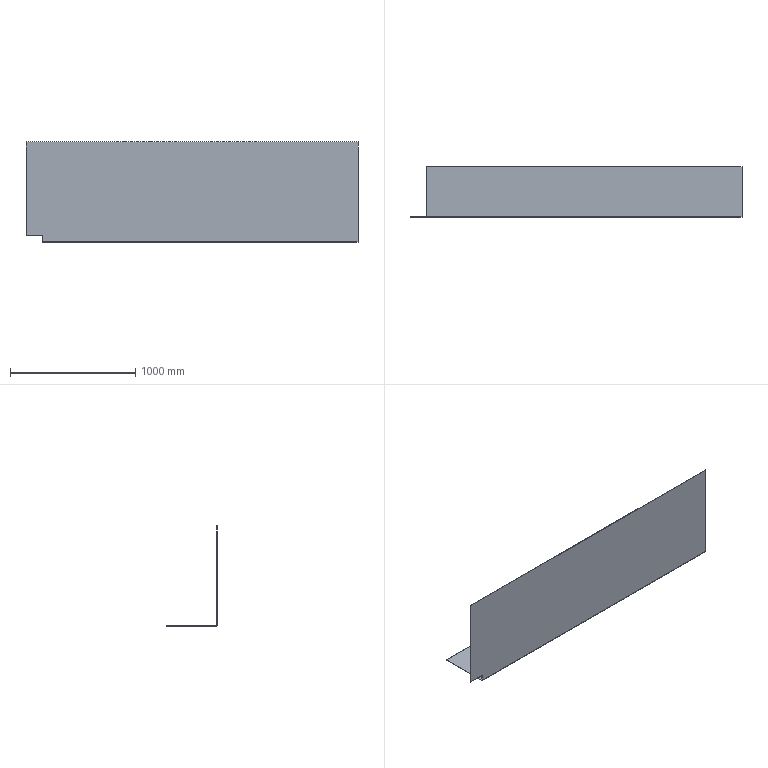Part | STEP file | E3-花纹Plate折弯1 | 1 solid | 14 faces | box 2648 x 403 x 798 mm | volume 9332526 mm3 | plane 12 | cylinder 2 | commonest cylinder face diameters 2 x1 8 x1
STEP:
#1=CARTESIAN_POINT('',(0.,0.,0.));
#2=DIRECTION('',(0.,0.,1.));
#3=DIRECTION('',(1.,0.,0.));
#4=AXIS2_PLACEMENT_3D('',#1,#2,#3);
#5=CARTESIAN_POINT('',(2648.,3.,-794.));
#6=VERTEX_POINT('',#5);
#7=CARTESIAN_POINT('',(2648.,3.,0.));
#8=VERTEX_POINT('',#7);
#9=CARTESIAN_POINT('',(2648.,3.,0.));
#10=DIRECTION('',(0.,0.,1.));
#11=VECTOR('',#10,1.);
#12=LINE('',#9,#11);
#13=CARTESIAN_POINT('',(2648.,3.,0.));
#14=DIRECTION('',(1.,0.,0.));
#15=DIRECTION('',(0.,0.,1.));
#16=AXIS2_PLACEMENT_3D('',#13,#14,#15);
#17=PLANE('',#16);
#18=CARTESIAN_POINT('',(0.,0.));
#19=DIRECTION('',(1.,0.));
#20=VECTOR('',#19,1.);
#21=LINE('',#18,#20);
#22=(GEOMETRIC_REPRESENTATION_CONTEXT(2)PARAMETRIC_REPRESENTATION_CONTEXT()REPRESENTATION_CONTEXT('',''));
#23=DEFINITIONAL_REPRESENTATION('',(#21),#22);
#24=PCURVE('',#17,#23);
#25=CARTESIAN_POINT('',(0.,3.,0.));
#26=DIRECTION('',(0.,1.,0.));
#27=DIRECTION('',(0.,0.,-1.));
#28=AXIS2_PLACEMENT_3D('',#25,#26,#27);
#29=PLANE('',#28);
#30=CARTESIAN_POINT('',(0.,-2648.));
#31=DIRECTION('',(-1.,0.));
#32=VECTOR('',#31,1.);
#33=LINE('',#30,#32);
#34=(GEOMETRIC_REPRESENTATION_CONTEXT(2)PARAMETRIC_REPRESENTATION_CONTEXT()REPRESENTATION_CONTEXT('',''));
#35=DEFINITIONAL_REPRESENTATION('',(#33),#34);
#36=PCURVE('',#29,#35);
#37=SURFACE_CURVE('',#12,(#24,#36),.PCURVE_S1.);
#38=EDGE_CURVE('',#6,#8,#37,.T.);
#39=ORIENTED_EDGE('',*,*,#38,.T.);
#40=CARTESIAN_POINT('',(2648.,0.,0.));
#41=VERTEX_POINT('',#40);
#42=CARTESIAN_POINT('',(2648.,3.,0.));
#43=DIRECTION('',(0.,1.,0.));
#44=VECTOR('',#43,1.);
#45=LINE('',#42,#44);
#46=CARTESIAN_POINT('',(0.,0.));
#47=DIRECTION('',(0.,-1.));
#48=VECTOR('',#47,1.);
#49=LINE('',#46,#48);
#50=(GEOMETRIC_REPRESENTATION_CONTEXT(2)PARAMETRIC_REPRESENTATION_CONTEXT()REPRESENTATION_CONTEXT('',''));
#51=DEFINITIONAL_REPRESENTATION('',(#49),#50);
#52=PCURVE('',#17,#51);
#53=CARTESIAN_POINT('',(0.,3.,0.));
#54=DIRECTION('',(0.,0.,1.));
#55=DIRECTION('',(-1.,0.,0.));
#56=AXIS2_PLACEMENT_3D('',#53,#54,#55);
#57=PLANE('',#56);
#58=CARTESIAN_POINT('',(-2648.,0.));
#59=DIRECTION('',(0.,-1.));
#60=VECTOR('',#59,1.);
#61=LINE('',#58,#60);
#62=(GEOMETRIC_REPRESENTATION_CONTEXT(2)PARAMETRIC_REPRESENTATION_CONTEXT()REPRESENTATION_CONTEXT('',''));
#63=DEFINITIONAL_REPRESENTATION('',(#61),#62);
#64=PCURVE('',#57,#63);
#65=SURFACE_CURVE('',#45,(#52,#64),.PCURVE_S1.);
#66=EDGE_CURVE('',#41,#8,#65,.T.);
#67=ORIENTED_EDGE('',*,*,#66,.F.);
#68=CARTESIAN_POINT('',(2648.,0.,-794.));
#69=VERTEX_POINT('',#68);
#70=CARTESIAN_POINT('',(2648.,0.,0.));
#71=DIRECTION('',(0.,0.,1.));
#72=VECTOR('',#71,1.);
#73=LINE('',#70,#72);
#74=CARTESIAN_POINT('',(0.,3.));
#75=DIRECTION('',(1.,0.));
#76=VECTOR('',#75,1.);
#77=LINE('',#74,#76);
#78=(GEOMETRIC_REPRESENTATION_CONTEXT(2)PARAMETRIC_REPRESENTATION_CONTEXT()REPRESENTATION_CONTEXT('',''));
#79=DEFINITIONAL_REPRESENTATION('',(#77),#78);
#80=PCURVE('',#17,#79);
#81=CARTESIAN_POINT('',(0.,0.,0.));
#82=DIRECTION('',(0.,1.,0.));
#83=DIRECTION('',(0.,0.,-1.));
#84=AXIS2_PLACEMENT_3D('',#81,#82,#83);
#85=PLANE('',#84);
#86=CARTESIAN_POINT('',(0.,-2648.));
#87=DIRECTION('',(-1.,0.));
#88=VECTOR('',#87,1.);
#89=LINE('',#86,#88);
#90=(GEOMETRIC_REPRESENTATION_CONTEXT(2)PARAMETRIC_REPRESENTATION_CONTEXT()REPRESENTATION_CONTEXT('',''));
#91=DEFINITIONAL_REPRESENTATION('',(#89),#90);
#92=PCURVE('',#85,#91);
#93=SURFACE_CURVE('',#73,(#80,#92),.PCURVE_S1.);
#94=EDGE_CURVE('',#69,#41,#93,.T.);
#95=ORIENTED_EDGE('',*,*,#94,.F.);
#96=CARTESIAN_POINT('',(2648.,3.,-794.));
#97=DIRECTION('',(0.,-1.,0.));
#98=VECTOR('',#97,1.);
#99=LINE('',#96,#98);
#100=CARTESIAN_POINT('',(-794.,0.));
#101=DIRECTION('',(0.,1.));
#102=VECTOR('',#101,1.);
#103=LINE('',#100,#102);
#104=(GEOMETRIC_REPRESENTATION_CONTEXT(2)PARAMETRIC_REPRESENTATION_CONTEXT()REPRESENTATION_CONTEXT('',''));
#105=DEFINITIONAL_REPRESENTATION('',(#103),#104);
#106=PCURVE('',#17,#105);
#107=CARTESIAN_POINT('',(2648.,4.,-794.));
#108=DIRECTION('',(-1.,0.,0.));
#109=DIRECTION('',(0.,0.,-1.));
#110=AXIS2_PLACEMENT_3D('',#107,#108,#109);
#111=PLANE('',#110);
#112=CARTESIAN_POINT('',(0.,1.));
#113=DIRECTION('',(0.,1.));
#114=VECTOR('',#113,1.);
#115=LINE('',#112,#114);
#116=(GEOMETRIC_REPRESENTATION_CONTEXT(2)PARAMETRIC_REPRESENTATION_CONTEXT()REPRESENTATION_CONTEXT('',''));
#117=DEFINITIONAL_REPRESENTATION('',(#115),#116);
#118=PCURVE('',#111,#117);
#119=SURFACE_CURVE('',#99,(#106,#118),.PCURVE_S1.);
#120=EDGE_CURVE('',#6,#69,#119,.T.);
#121=ORIENTED_EDGE('',*,*,#120,.F.);
#122=EDGE_LOOP('',(#39,#67,#95,#121));
#123=FACE_BOUND('',#122,.T.);
#124=ADVANCED_FACE('',(#123),#17,.T.);
#125=CARTESIAN_POINT('',(130.,3.,-746.));
#126=VERTEX_POINT('',#125);
#127=CARTESIAN_POINT('',(0.,3.,-746.));
#128=VERTEX_POINT('',#127);
#129=CARTESIAN_POINT('',(0.,3.,-746.));
#130=DIRECTION('',(-1.,0.,0.));
#131=VECTOR('',#130,1.);
#132=LINE('',#129,#131);
#133=CARTESIAN_POINT('',(746.,0.));
#134=DIRECTION('',(0.,1.));
#135=VECTOR('',#134,1.);
#136=LINE('',#133,#135);
#137=(GEOMETRIC_REPRESENTATION_CONTEXT(2)PARAMETRIC_REPRESENTATION_CONTEXT()REPRESENTATION_CONTEXT('',''));
#138=DEFINITIONAL_REPRESENTATION('',(#136),#137);
#139=PCURVE('',#29,#138);
#140=CARTESIAN_POINT('',(0.,-497.,-746.));
#141=DIRECTION('',(0.,0.,1.));
#142=DIRECTION('',(-1.,0.,0.));
#143=AXIS2_PLACEMENT_3D('',#140,#141,#142);
#144=PLANE('',#143);
#145=CARTESIAN_POINT('',(0.,-500.));
#146=DIRECTION('',(1.,0.));
#147=VECTOR('',#146,1.);
#148=LINE('',#145,#147);
#149=(GEOMETRIC_REPRESENTATION_CONTEXT(2)PARAMETRIC_REPRESENTATION_CONTEXT()REPRESENTATION_CONTEXT('',''));
#150=DEFINITIONAL_REPRESENTATION('',(#148),#149);
#151=PCURVE('',#144,#150);
#152=SURFACE_CURVE('',#132,(#139,#151),.PCURVE_S1.);
#153=EDGE_CURVE('',#126,#128,#152,.T.);
#154=ORIENTED_EDGE('',*,*,#153,.T.);
#155=CARTESIAN_POINT('',(0.,3.,0.));
#156=VERTEX_POINT('',#155);
#157=CARTESIAN_POINT('',(0.,3.,0.));
#158=DIRECTION('',(0.,0.,-1.));
#159=VECTOR('',#158,1.);
#160=LINE('',#157,#159);
#161=CARTESIAN_POINT('',(0.,0.));
#162=DIRECTION('',(1.,0.));
#163=VECTOR('',#162,1.);
#164=LINE('',#161,#163);
#165=(GEOMETRIC_REPRESENTATION_CONTEXT(2)PARAMETRIC_REPRESENTATION_CONTEXT()REPRESENTATION_CONTEXT('',''));
#166=DEFINITIONAL_REPRESENTATION('',(#164),#165);
#167=PCURVE('',#29,#166);
#168=CARTESIAN_POINT('',(0.,3.,0.));
#169=DIRECTION('',(-1.,0.,0.));
#170=DIRECTION('',(0.,0.,-1.));
#171=AXIS2_PLACEMENT_3D('',#168,#169,#170);
#172=PLANE('',#171);
#173=CARTESIAN_POINT('',(0.,0.));
#174=DIRECTION('',(1.,0.));
#175=VECTOR('',#174,1.);
#176=LINE('',#173,#175);
#177=(GEOMETRIC_REPRESENTATION_CONTEXT(2)PARAMETRIC_REPRESENTATION_CONTEXT()REPRESENTATION_CONTEXT('',''));
#178=DEFINITIONAL_REPRESENTATION('',(#176),#177);
#179=PCURVE('',#172,#178);
#180=SURFACE_CURVE('',#160,(#167,#179),.PCURVE_S1.);
#181=EDGE_CURVE('',#156,#128,#180,.T.);
#182=ORIENTED_EDGE('',*,*,#181,.F.);
#183=CARTESIAN_POINT('',(0.,3.,0.));
#184=DIRECTION('',(-1.,0.,0.));
#185=VECTOR('',#184,1.);
#186=LINE('',#183,#185);
#187=CARTESIAN_POINT('',(0.,0.));
#188=DIRECTION('',(0.,1.));
#189=VECTOR('',#188,1.);
#190=LINE('',#187,#189);
#191=(GEOMETRIC_REPRESENTATION_CONTEXT(2)PARAMETRIC_REPRESENTATION_CONTEXT()REPRESENTATION_CONTEXT('',''));
#192=DEFINITIONAL_REPRESENTATION('',(#190),#191);
#193=PCURVE('',#29,#192);
#194=CARTESIAN_POINT('',(0.,0.));
#195=DIRECTION('',(1.,0.));
#196=VECTOR('',#195,1.);
#197=LINE('',#194,#196);
#198=(GEOMETRIC_REPRESENTATION_CONTEXT(2)PARAMETRIC_REPRESENTATION_CONTEXT()REPRESENTATION_CONTEXT('',''));
#199=DEFINITIONAL_REPRESENTATION('',(#197),#198);
#200=PCURVE('',#57,#199);
#201=SURFACE_CURVE('',#186,(#193,#200),.PCURVE_S1.);
#202=EDGE_CURVE('',#8,#156,#201,.T.);
#203=ORIENTED_EDGE('',*,*,#202,.F.);
#204=ORIENTED_EDGE('',*,*,#38,.F.);
#205=CARTESIAN_POINT('',(130.,3.,-794.));
#206=VERTEX_POINT('',#205);
#207=CARTESIAN_POINT('',(2648.,3.,-794.));
#208=DIRECTION('',(-1.,0.,0.));
#209=VECTOR('',#208,1.);
#210=LINE('',#207,#209);
#211=CARTESIAN_POINT('',(794.,-2648.));
#212=DIRECTION('',(0.,1.));
#213=VECTOR('',#212,1.);
#214=LINE('',#211,#213);
#215=(GEOMETRIC_REPRESENTATION_CONTEXT(2)PARAMETRIC_REPRESENTATION_CONTEXT()REPRESENTATION_CONTEXT('',''));
#216=DEFINITIONAL_REPRESENTATION('',(#214),#215);
#217=PCURVE('',#29,#216);
#218=CARTESIAN_POINT('',(2648.,4.,-794.));
#219=DIRECTION('',(1.,0.,0.));
#220=DIRECTION('',(0.,0.,-1.));
#221=AXIS2_PLACEMENT_3D('',#218,#219,#220);
#222=CYLINDRICAL_SURFACE('',#221,1.);
#223=CARTESIAN_POINT('',(4.712,0.));
#224=DIRECTION('',(0.,-1.));
#225=VECTOR('',#224,1.);
#226=LINE('',#223,#225);
#227=(GEOMETRIC_REPRESENTATION_CONTEXT(2)PARAMETRIC_REPRESENTATION_CONTEXT()REPRESENTATION_CONTEXT('',''));
#228=DEFINITIONAL_REPRESENTATION('',(#226),#227);
#229=PCURVE('',#222,#228);
#230=SURFACE_CURVE('',#210,(#217,#229),.PCURVE_S1.);
#231=EDGE_CURVE('',#6,#206,#230,.T.);
#232=ORIENTED_EDGE('',*,*,#231,.T.);
#233=CARTESIAN_POINT('',(130.,3.,0.));
#234=DIRECTION('',(0.,0.,1.));
#235=VECTOR('',#234,1.);
#236=LINE('',#233,#235);
#237=CARTESIAN_POINT('',(0.,-130.));
#238=DIRECTION('',(-1.,0.));
#239=VECTOR('',#238,1.);
#240=LINE('',#237,#239);
#241=(GEOMETRIC_REPRESENTATION_CONTEXT(2)PARAMETRIC_REPRESENTATION_CONTEXT()REPRESENTATION_CONTEXT('',''));
#242=DEFINITIONAL_REPRESENTATION('',(#240),#241);
#243=PCURVE('',#29,#242);
#244=CARTESIAN_POINT('',(130.,-497.,-746.));
#245=DIRECTION('',(1.,0.,0.));
#246=DIRECTION('',(0.,0.,1.));
#247=AXIS2_PLACEMENT_3D('',#244,#245,#246);
#248=PLANE('',#247);
#249=CARTESIAN_POINT('',(746.,-500.));
#250=DIRECTION('',(1.,0.));
#251=VECTOR('',#250,1.);
#252=LINE('',#249,#251);
#253=(GEOMETRIC_REPRESENTATION_CONTEXT(2)PARAMETRIC_REPRESENTATION_CONTEXT()REPRESENTATION_CONTEXT('',''));
#254=DEFINITIONAL_REPRESENTATION('',(#252),#253);
#255=PCURVE('',#248,#254);
#256=SURFACE_CURVE('',#236,(#243,#255),.PCURVE_S1.);
#257=EDGE_CURVE('',#206,#126,#256,.T.);
#258=ORIENTED_EDGE('',*,*,#257,.T.);
#259=EDGE_LOOP('',(#154,#182,#203,#204,#232,#258));
#260=FACE_BOUND('',#259,.T.);
#261=ADVANCED_FACE('',(#260),#29,.T.);
#262=CARTESIAN_POINT('',(130.,0.,-794.));
#263=VERTEX_POINT('',#262);
#264=CARTESIAN_POINT('',(130.,0.,-746.));
#265=VERTEX_POINT('',#264);
#266=CARTESIAN_POINT('',(130.,0.,0.));
#267=DIRECTION('',(0.,0.,1.));
#268=VECTOR('',#267,1.);
#269=LINE('',#266,#268);
#270=CARTESIAN_POINT('',(0.,-130.));
#271=DIRECTION('',(-1.,0.));
#272=VECTOR('',#271,1.);
#273=LINE('',#270,#272);
#274=(GEOMETRIC_REPRESENTATION_CONTEXT(2)PARAMETRIC_REPRESENTATION_CONTEXT()REPRESENTATION_CONTEXT('',''));
#275=DEFINITIONAL_REPRESENTATION('',(#273),#274);
#276=PCURVE('',#85,#275);
#277=CARTESIAN_POINT('',(746.,-497.));
#278=DIRECTION('',(1.,0.));
#279=VECTOR('',#278,1.);
#280=LINE('',#277,#279);
#281=(GEOMETRIC_REPRESENTATION_CONTEXT(2)PARAMETRIC_REPRESENTATION_CONTEXT()REPRESENTATION_CONTEXT('',''));
#282=DEFINITIONAL_REPRESENTATION('',(#280),#281);
#283=PCURVE('',#248,#282);
#284=SURFACE_CURVE('',#269,(#276,#283),.PCURVE_S1.);
#285=EDGE_CURVE('',#263,#265,#284,.T.);
#286=ORIENTED_EDGE('',*,*,#285,.F.);
#287=CARTESIAN_POINT('',(2648.,0.,-794.));
#288=DIRECTION('',(-1.,0.,0.));
#289=VECTOR('',#288,1.);
#290=LINE('',#287,#289);
#291=CARTESIAN_POINT('',(794.,-2648.));
#292=DIRECTION('',(0.,1.));
#293=VECTOR('',#292,1.);
#294=LINE('',#291,#293);
#295=(GEOMETRIC_REPRESENTATION_CONTEXT(2)PARAMETRIC_REPRESENTATION_CONTEXT()REPRESENTATION_CONTEXT('',''));
#296=DEFINITIONAL_REPRESENTATION('',(#294),#295);
#297=PCURVE('',#85,#296);
#298=CARTESIAN_POINT('',(2648.,4.,-794.));
#299=DIRECTION('',(1.,0.,0.));
#300=DIRECTION('',(0.,0.,-1.));
#301=AXIS2_PLACEMENT_3D('',#298,#299,#300);
#302=CYLINDRICAL_SURFACE('',#301,4.);
#303=CARTESIAN_POINT('',(4.712,0.));
#304=DIRECTION('',(0.,-1.));
#305=VECTOR('',#304,1.);
#306=LINE('',#303,#305);
#307=(GEOMETRIC_REPRESENTATION_CONTEXT(2)PARAMETRIC_REPRESENTATION_CONTEXT()REPRESENTATION_CONTEXT('',''));
#308=DEFINITIONAL_REPRESENTATION('',(#306),#307);
#309=PCURVE('',#302,#308);
#310=SURFACE_CURVE('',#290,(#297,#309),.PCURVE_S1.);
#311=EDGE_CURVE('',#69,#263,#310,.T.);
#312=ORIENTED_EDGE('',*,*,#311,.F.);
#313=ORIENTED_EDGE('',*,*,#94,.T.);
#314=CARTESIAN_POINT('',(0.,0.,0.));
#315=VERTEX_POINT('',#314);
#316=CARTESIAN_POINT('',(0.,0.,0.));
#317=DIRECTION('',(-1.,0.,0.));
#318=VECTOR('',#317,1.);
#319=LINE('',#316,#318);
#320=CARTESIAN_POINT('',(0.,0.));
#321=DIRECTION('',(0.,1.));
#322=VECTOR('',#321,1.);
#323=LINE('',#320,#322);
#324=(GEOMETRIC_REPRESENTATION_CONTEXT(2)PARAMETRIC_REPRESENTATION_CONTEXT()REPRESENTATION_CONTEXT('',''));
#325=DEFINITIONAL_REPRESENTATION('',(#323),#324);
#326=PCURVE('',#85,#325);
#327=CARTESIAN_POINT('',(0.,3.));
#328=DIRECTION('',(1.,0.));
#329=VECTOR('',#328,1.);
#330=LINE('',#327,#329);
#331=(GEOMETRIC_REPRESENTATION_CONTEXT(2)PARAMETRIC_REPRESENTATION_CONTEXT()REPRESENTATION_CONTEXT('',''));
#332=DEFINITIONAL_REPRESENTATION('',(#330),#331);
#333=PCURVE('',#57,#332);
#334=SURFACE_CURVE('',#319,(#326,#333),.PCURVE_S1.);
#335=EDGE_CURVE('',#41,#315,#334,.T.);
#336=ORIENTED_EDGE('',*,*,#335,.T.);
#337=CARTESIAN_POINT('',(0.,0.,-746.));
#338=VERTEX_POINT('',#337);
#339=CARTESIAN_POINT('',(0.,0.,0.));
#340=DIRECTION('',(0.,0.,-1.));
#341=VECTOR('',#340,1.);
#342=LINE('',#339,#341);
#343=CARTESIAN_POINT('',(0.,0.));
#344=DIRECTION('',(1.,0.));
#345=VECTOR('',#344,1.);
#346=LINE('',#343,#345);
#347=(GEOMETRIC_REPRESENTATION_CONTEXT(2)PARAMETRIC_REPRESENTATION_CONTEXT()REPRESENTATION_CONTEXT('',''));
#348=DEFINITIONAL_REPRESENTATION('',(#346),#347);
#349=PCURVE('',#85,#348);
#350=CARTESIAN_POINT('',(0.,3.));
#351=DIRECTION('',(1.,0.));
#352=VECTOR('',#351,1.);
#353=LINE('',#350,#352);
#354=(GEOMETRIC_REPRESENTATION_CONTEXT(2)PARAMETRIC_REPRESENTATION_CONTEXT()REPRESENTATION_CONTEXT('',''));
#355=DEFINITIONAL_REPRESENTATION('',(#353),#354);
#356=PCURVE('',#172,#355);
#357=SURFACE_CURVE('',#342,(#349,#356),.PCURVE_S1.);
#358=EDGE_CURVE('',#315,#338,#357,.T.);
#359=ORIENTED_EDGE('',*,*,#358,.T.);
#360=CARTESIAN_POINT('',(0.,0.,-746.));
#361=DIRECTION('',(-1.,0.,0.));
#362=VECTOR('',#361,1.);
#363=LINE('',#360,#362);
#364=CARTESIAN_POINT('',(746.,0.));
#365=DIRECTION('',(0.,1.));
#366=VECTOR('',#365,1.);
#367=LINE('',#364,#366);
#368=(GEOMETRIC_REPRESENTATION_CONTEXT(2)PARAMETRIC_REPRESENTATION_CONTEXT()REPRESENTATION_CONTEXT('',''));
#369=DEFINITIONAL_REPRESENTATION('',(#367),#368);
#370=PCURVE('',#85,#369);
#371=CARTESIAN_POINT('',(0.,-497.));
#372=DIRECTION('',(1.,0.));
#373=VECTOR('',#372,1.);
#374=LINE('',#371,#373);
#375=(GEOMETRIC_REPRESENTATION_CONTEXT(2)PARAMETRIC_REPRESENTATION_CONTEXT()REPRESENTATION_CONTEXT('',''));
#376=DEFINITIONAL_REPRESENTATION('',(#374),#375);
#377=PCURVE('',#144,#376);
#378=SURFACE_CURVE('',#363,(#370,#377),.PCURVE_S1.);
#379=EDGE_CURVE('',#265,#338,#378,.T.);
#380=ORIENTED_EDGE('',*,*,#379,.F.);
#381=EDGE_LOOP('',(#286,#312,#313,#336,#359,#380));
#382=FACE_BOUND('',#381,.T.);
#383=ADVANCED_FACE('',(#382),#85,.F.);
#384=ORIENTED_EDGE('',*,*,#66,.T.);
#385=ORIENTED_EDGE('',*,*,#202,.T.);
#386=CARTESIAN_POINT('',(0.,3.,0.));
#387=DIRECTION('',(0.,1.,0.));
#388=VECTOR('',#387,1.);
#389=LINE('',#386,#388);
#390=CARTESIAN_POINT('',(0.,0.));
#391=DIRECTION('',(0.,-1.));
#392=VECTOR('',#391,1.);
#393=LINE('',#390,#392);
#394=(GEOMETRIC_REPRESENTATION_CONTEXT(2)PARAMETRIC_REPRESENTATION_CONTEXT()REPRESENTATION_CONTEXT('',''));
#395=DEFINITIONAL_REPRESENTATION('',(#393),#394);
#396=PCURVE('',#57,#395);
#397=CARTESIAN_POINT('',(0.,0.));
#398=DIRECTION('',(0.,-1.));
#399=VECTOR('',#398,1.);
#400=LINE('',#397,#399);
#401=(GEOMETRIC_REPRESENTATION_CONTEXT(2)PARAMETRIC_REPRESENTATION_CONTEXT()REPRESENTATION_CONTEXT('',''));
#402=DEFINITIONAL_REPRESENTATION('',(#400),#401);
#403=PCURVE('',#172,#402);
#404=SURFACE_CURVE('',#389,(#396,#403),.PCURVE_S1.);
#405=EDGE_CURVE('',#315,#156,#404,.T.);
#406=ORIENTED_EDGE('',*,*,#405,.F.);
#407=ORIENTED_EDGE('',*,*,#335,.F.);
#408=EDGE_LOOP('',(#384,#385,#406,#407));
#409=FACE_BOUND('',#408,.T.);
#410=ADVANCED_FACE('',(#409),#57,.T.);
#411=CARTESIAN_POINT('',(0.,-497.,-746.));
#412=DIRECTION('',(0.,1.,0.));
#413=VECTOR('',#412,1.);
#414=LINE('',#411,#413);
#415=CARTESIAN_POINT('',(746.,500.));
#416=DIRECTION('',(0.,-1.));
#417=VECTOR('',#416,1.);
#418=LINE('',#415,#417);
#419=(GEOMETRIC_REPRESENTATION_CONTEXT(2)PARAMETRIC_REPRESENTATION_CONTEXT()REPRESENTATION_CONTEXT('',''));
#420=DEFINITIONAL_REPRESENTATION('',(#418),#419);
#421=PCURVE('',#172,#420);
#422=CARTESIAN_POINT('',(0.,0.));
#423=DIRECTION('',(0.,-1.));
#424=VECTOR('',#423,1.);
#425=LINE('',#422,#424);
#426=(GEOMETRIC_REPRESENTATION_CONTEXT(2)PARAMETRIC_REPRESENTATION_CONTEXT()REPRESENTATION_CONTEXT('',''));
#427=DEFINITIONAL_REPRESENTATION('',(#425),#426);
#428=PCURVE('',#144,#427);
#429=SURFACE_CURVE('',#414,(#421,#428),.PCURVE_S1.);
#430=EDGE_CURVE('',#338,#128,#429,.T.);
#431=ORIENTED_EDGE('',*,*,#430,.F.);
#432=ORIENTED_EDGE('',*,*,#358,.F.);
#433=ORIENTED_EDGE('',*,*,#405,.T.);
#434=ORIENTED_EDGE('',*,*,#181,.T.);
#435=EDGE_LOOP('',(#431,#432,#433,#434));
#436=FACE_BOUND('',#435,.T.);
#437=ADVANCED_FACE('',(#436),#172,.T.);
#438=CARTESIAN_POINT('',(2648.,4.,-795.));
#439=VERTEX_POINT('',#438);
#440=CARTESIAN_POINT('',(2648.,4.,-794.));
#441=DIRECTION('',(-1.,0.,0.));
#442=DIRECTION('',(0.,0.,1.));
#443=AXIS2_PLACEMENT_3D('',#440,#441,#442);
#444=CIRCLE('',#443,1.);
#445=CARTESIAN_POINT('',(0.,0.));
#446=DIRECTION('',(-1.,0.));
#447=AXIS2_PLACEMENT_2D('',#445,#446);
#448=CIRCLE('',#447,1.);
#449=(GEOMETRIC_REPRESENTATION_CONTEXT(2)PARAMETRIC_REPRESENTATION_CONTEXT()REPRESENTATION_CONTEXT('',''));
#450=DEFINITIONAL_REPRESENTATION('',(#448),#449);
#451=PCURVE('',#111,#450);
#452=CARTESIAN_POINT('',(9.425,0.));
#453=DIRECTION('',(-1.,0.));
#454=VECTOR('',#453,1.);
#455=LINE('',#452,#454);
#456=(GEOMETRIC_REPRESENTATION_CONTEXT(2)PARAMETRIC_REPRESENTATION_CONTEXT()REPRESENTATION_CONTEXT('',''));
#457=DEFINITIONAL_REPRESENTATION('',(#455),#456);
#458=PCURVE('',#222,#457);
#459=SURFACE_CURVE('',#444,(#451,#458),.PCURVE_S1.);
#460=EDGE_CURVE('',#439,#6,#459,.T.);
#461=ORIENTED_EDGE('',*,*,#460,.T.);
#462=ORIENTED_EDGE('',*,*,#120,.T.);
#463=CARTESIAN_POINT('',(2648.,4.,-798.));
#464=VERTEX_POINT('',#463);
#465=CARTESIAN_POINT('',(2648.,4.,-794.));
#466=DIRECTION('',(-1.,0.,0.));
#467=DIRECTION('',(0.,0.,1.));
#468=AXIS2_PLACEMENT_3D('',#465,#466,#467);
#469=CIRCLE('',#468,4.);
#470=CARTESIAN_POINT('',(0.,0.));
#471=DIRECTION('',(-1.,0.));
#472=AXIS2_PLACEMENT_2D('',#470,#471);
#473=CIRCLE('',#472,4.);
#474=(GEOMETRIC_REPRESENTATION_CONTEXT(2)PARAMETRIC_REPRESENTATION_CONTEXT()REPRESENTATION_CONTEXT('',''));
#475=DEFINITIONAL_REPRESENTATION('',(#473),#474);
#476=PCURVE('',#111,#475);
#477=CARTESIAN_POINT('',(9.425,0.));
#478=DIRECTION('',(-1.,0.));
#479=VECTOR('',#478,1.);
#480=LINE('',#477,#479);
#481=(GEOMETRIC_REPRESENTATION_CONTEXT(2)PARAMETRIC_REPRESENTATION_CONTEXT()REPRESENTATION_CONTEXT('',''));
#482=DEFINITIONAL_REPRESENTATION('',(#480),#481);
#483=PCURVE('',#302,#482);
#484=SURFACE_CURVE('',#469,(#476,#483),.PCURVE_S1.);
#485=EDGE_CURVE('',#464,#69,#484,.T.);
#486=ORIENTED_EDGE('',*,*,#485,.F.);
#487=CARTESIAN_POINT('',(2648.,4.,-795.));
#488=DIRECTION('',(0.,0.,-1.));
#489=VECTOR('',#488,1.);
#490=LINE('',#487,#489);
#491=CARTESIAN_POINT('',(1.,0.));
#492=DIRECTION('',(1.,0.));
#493=VECTOR('',#492,1.);
#494=LINE('',#491,#493);
#495=(GEOMETRIC_REPRESENTATION_CONTEXT(2)PARAMETRIC_REPRESENTATION_CONTEXT()REPRESENTATION_CONTEXT('',''));
#496=DEFINITIONAL_REPRESENTATION('',(#494),#495);
#497=PCURVE('',#111,#496);
#498=CARTESIAN_POINT('',(2648.,403.,-798.));
#499=DIRECTION('',(-1.,0.,0.));
#500=DIRECTION('',(0.,0.,-1.));
#501=AXIS2_PLACEMENT_3D('',#498,#499,#500);
#502=PLANE('',#501);
#503=CARTESIAN_POINT('',(-3.,399.));
#504=DIRECTION('',(1.,0.));
#505=VECTOR('',#504,1.);
#506=LINE('',#503,#505);
#507=(GEOMETRIC_REPRESENTATION_CONTEXT(2)PARAMETRIC_REPRESENTATION_CONTEXT()REPRESENTATION_CONTEXT('',''));
#508=DEFINITIONAL_REPRESENTATION('',(#506),#507);
#509=PCURVE('',#502,#508);
#510=SURFACE_CURVE('',#490,(#497,#509),.PCURVE_S1.);
#511=EDGE_CURVE('',#439,#464,#510,.T.);
#512=ORIENTED_EDGE('',*,*,#511,.F.);
#513=EDGE_LOOP('',(#461,#462,#486,#512));
#514=FACE_BOUND('',#513,.T.);
#515=ADVANCED_FACE('',(#514),#111,.F.);
#516=CARTESIAN_POINT('',(130.,4.,-798.));
#517=VERTEX_POINT('',#516);
#518=CARTESIAN_POINT('',(130.,4.,-794.));
#519=DIRECTION('',(1.,0.,0.));
#520=DIRECTION('',(0.,0.,1.));
#521=AXIS2_PLACEMENT_3D('',#518,#519,#520);
#522=CIRCLE('',#521,4.);
#523=CARTESIAN_POINT('',(3.142,-2518.));
#524=DIRECTION('',(1.,0.));
#525=VECTOR('',#524,1.);
#526=LINE('',#523,#525);
#527=(GEOMETRIC_REPRESENTATION_CONTEXT(2)PARAMETRIC_REPRESENTATION_CONTEXT()REPRESENTATION_CONTEXT('',''));
#528=DEFINITIONAL_REPRESENTATION('',(#526),#527);
#529=PCURVE('',#302,#528);
#530=CARTESIAN_POINT('',(-48.,-501.));
#531=DIRECTION('',(1.,0.));
#532=AXIS2_PLACEMENT_2D('',#530,#531);
#533=CIRCLE('',#532,4.);
#534=(GEOMETRIC_REPRESENTATION_CONTEXT(2)PARAMETRIC_REPRESENTATION_CONTEXT()REPRESENTATION_CONTEXT('',''));
#535=DEFINITIONAL_REPRESENTATION('',(#533),#534);
#536=PCURVE('',#248,#535);
#537=SURFACE_CURVE('',#522,(#529,#536),.PCURVE_S1.);
#538=EDGE_CURVE('',#263,#517,#537,.T.);
#539=ORIENTED_EDGE('',*,*,#538,.T.);
#540=CARTESIAN_POINT('',(0.,4.,-798.));
#541=DIRECTION('',(-1.,0.,0.));
#542=VECTOR('',#541,1.);
#543=LINE('',#540,#542);
#544=CARTESIAN_POINT('',(6.283,-2648.));
#545=DIRECTION('',(0.,-1.));
#546=VECTOR('',#545,1.);
#547=LINE('',#544,#546);
#548=(GEOMETRIC_REPRESENTATION_CONTEXT(2)PARAMETRIC_REPRESENTATION_CONTEXT()REPRESENTATION_CONTEXT('',''));
#549=DEFINITIONAL_REPRESENTATION('',(#547),#548);
#550=PCURVE('',#302,#549);
#551=CARTESIAN_POINT('',(0.,0.,-798.));
#552=DIRECTION('',(0.,0.,1.));
#553=DIRECTION('',(-1.,0.,0.));
#554=AXIS2_PLACEMENT_3D('',#551,#552,#553);
#555=PLANE('',#554);
#556=CARTESIAN_POINT('',(0.,-4.));
#557=DIRECTION('',(1.,0.));
#558=VECTOR('',#557,1.);
#559=LINE('',#556,#558);
#560=(GEOMETRIC_REPRESENTATION_CONTEXT(2)PARAMETRIC_REPRESENTATION_CONTEXT()REPRESENTATION_CONTEXT('',''));
#561=DEFINITIONAL_REPRESENTATION('',(#559),#560);
#562=PCURVE('',#555,#561);
#563=SURFACE_CURVE('',#543,(#550,#562),.PCURVE_S1.);
#564=EDGE_CURVE('',#464,#517,#563,.T.);
#565=ORIENTED_EDGE('',*,*,#564,.F.);
#566=ORIENTED_EDGE('',*,*,#485,.T.);
#567=ORIENTED_EDGE('',*,*,#311,.T.);
#568=EDGE_LOOP('',(#539,#565,#566,#567));
#569=FACE_BOUND('',#568,.T.);
#570=ADVANCED_FACE('',(#569),#302,.T.);
#571=CARTESIAN_POINT('',(130.,4.,-795.));
#572=VERTEX_POINT('',#571);
#573=CARTESIAN_POINT('',(130.,4.,-794.));
#574=DIRECTION('',(1.,0.,0.));
#575=DIRECTION('',(0.,0.,1.));
#576=AXIS2_PLACEMENT_3D('',#573,#574,#575);
#577=CIRCLE('',#576,1.);
#578=CARTESIAN_POINT('',(3.142,-2518.));
#579=DIRECTION('',(1.,0.));
#580=VECTOR('',#579,1.);
#581=LINE('',#578,#580);
#582=(GEOMETRIC_REPRESENTATION_CONTEXT(2)PARAMETRIC_REPRESENTATION_CONTEXT()REPRESENTATION_CONTEXT('',''));
#583=DEFINITIONAL_REPRESENTATION('',(#581),#582);
#584=PCURVE('',#222,#583);
#585=CARTESIAN_POINT('',(-48.,-501.));
#586=DIRECTION('',(1.,0.));
#587=AXIS2_PLACEMENT_2D('',#585,#586);
#588=CIRCLE('',#587,1.);
#589=(GEOMETRIC_REPRESENTATION_CONTEXT(2)PARAMETRIC_REPRESENTATION_CONTEXT()REPRESENTATION_CONTEXT('',''));
#590=DEFINITIONAL_REPRESENTATION('',(#588),#589);
#591=PCURVE('',#248,#590);
#592=SURFACE_CURVE('',#577,(#584,#591),.PCURVE_S1.);
#593=EDGE_CURVE('',#206,#572,#592,.T.);
#594=ORIENTED_EDGE('',*,*,#593,.T.);
#595=CARTESIAN_POINT('',(0.,4.,-795.));
#596=DIRECTION('',(1.,0.,0.));
#597=VECTOR('',#596,1.);
#598=LINE('',#595,#597);
#599=CARTESIAN_POINT('',(6.283,-2648.));
#600=DIRECTION('',(0.,1.));
#601=VECTOR('',#600,1.);
#602=LINE('',#599,#601);
#603=(GEOMETRIC_REPRESENTATION_CONTEXT(2)PARAMETRIC_REPRESENTATION_CONTEXT()REPRESENTATION_CONTEXT('',''));
#604=DEFINITIONAL_REPRESENTATION('',(#602),#603);
#605=PCURVE('',#222,#604);
#606=CARTESIAN_POINT('',(0.,0.,-795.));
#607=DIRECTION('',(0.,0.,1.));
#608=DIRECTION('',(-1.,0.,0.));
#609=AXIS2_PLACEMENT_3D('',#606,#607,#608);
#610=PLANE('',#609);
#611=CARTESIAN_POINT('',(0.,-4.));
#612=DIRECTION('',(-1.,0.));
#613=VECTOR('',#612,1.);
#614=LINE('',#611,#613);
#615=(GEOMETRIC_REPRESENTATION_CONTEXT(2)PARAMETRIC_REPRESENTATION_CONTEXT()REPRESENTATION_CONTEXT('',''));
#616=DEFINITIONAL_REPRESENTATION('',(#614),#615);
#617=PCURVE('',#610,#616);
#618=SURFACE_CURVE('',#598,(#605,#617),.PCURVE_S1.);
#619=EDGE_CURVE('',#572,#439,#618,.T.);
#620=ORIENTED_EDGE('',*,*,#619,.T.);
#621=ORIENTED_EDGE('',*,*,#460,.T.);
#622=ORIENTED_EDGE('',*,*,#231,.T.);
#623=EDGE_LOOP('',(#594,#620,#621,#622));
#624=FACE_BOUND('',#623,.F.);
#625=ADVANCED_FACE('',(#624),#222,.F.);
#626=ORIENTED_EDGE('',*,*,#511,.T.);
#627=CARTESIAN_POINT('',(2648.,403.,-798.));
#628=VERTEX_POINT('',#627);
#629=CARTESIAN_POINT('',(2648.,0.,-798.));
#630=DIRECTION('',(0.,1.,0.));
#631=VECTOR('',#630,1.);
#632=LINE('',#629,#631);
#633=CARTESIAN_POINT('',(0.,403.));
#634=DIRECTION('',(0.,-1.));
#635=VECTOR('',#634,1.);
#636=LINE('',#633,#635);
#637=(GEOMETRIC_REPRESENTATION_CONTEXT(2)PARAMETRIC_REPRESENTATION_CONTEXT()REPRESENTATION_CONTEXT('',''));
#638=DEFINITIONAL_REPRESENTATION('',(#636),#637);
#639=PCURVE('',#502,#638);
#640=CARTESIAN_POINT('',(-2648.,0.));
#641=DIRECTION('',(0.,-1.));
#642=VECTOR('',#641,1.);
#643=LINE('',#640,#642);
#644=(GEOMETRIC_REPRESENTATION_CONTEXT(2)PARAMETRIC_REPRESENTATION_CONTEXT()REPRESENTATION_CONTEXT('',''));
#645=DEFINITIONAL_REPRESENTATION('',(#643),#644);
#646=PCURVE('',#555,#645);
#647=SURFACE_CURVE('',#632,(#639,#646),.PCURVE_S1.);
#648=EDGE_CURVE('',#464,#628,#647,.T.);
#649=ORIENTED_EDGE('',*,*,#648,.T.);
#650=CARTESIAN_POINT('',(2648.,403.,-795.));
#651=VERTEX_POINT('',#650);
#652=CARTESIAN_POINT('',(2648.,403.,-798.));
#653=DIRECTION('',(0.,0.,1.));
#654=VECTOR('',#653,1.);
#655=LINE('',#652,#654);
#656=CARTESIAN_POINT('',(0.,0.));
#657=DIRECTION('',(-1.,0.));
#658=VECTOR('',#657,1.);
#659=LINE('',#656,#658);
#660=(GEOMETRIC_REPRESENTATION_CONTEXT(2)PARAMETRIC_REPRESENTATION_CONTEXT()REPRESENTATION_CONTEXT('',''));
#661=DEFINITIONAL_REPRESENTATION('',(#659),#660);
#662=PCURVE('',#502,#661);
#663=CARTESIAN_POINT('',(0.,403.,-798.));
#664=DIRECTION('',(0.,-1.,0.));
#665=DIRECTION('',(0.,0.,1.));
#666=AXIS2_PLACEMENT_3D('',#663,#664,#665);
#667=PLANE('',#666);
#668=CARTESIAN_POINT('',(0.,-2648.));
#669=DIRECTION('',(1.,0.));
#670=VECTOR('',#669,1.);
#671=LINE('',#668,#670);
#672=(GEOMETRIC_REPRESENTATION_CONTEXT(2)PARAMETRIC_REPRESENTATION_CONTEXT()REPRESENTATION_CONTEXT('',''));
#673=DEFINITIONAL_REPRESENTATION('',(#671),#672);
#674=PCURVE('',#667,#673);
#675=SURFACE_CURVE('',#655,(#662,#674),.PCURVE_S1.);
#676=EDGE_CURVE('',#628,#651,#675,.T.);
#677=ORIENTED_EDGE('',*,*,#676,.T.);
#678=CARTESIAN_POINT('',(2648.,403.,-795.));
#679=DIRECTION('',(0.,1.,0.));
#680=VECTOR('',#679,1.);
#681=LINE('',#678,#680);
#682=CARTESIAN_POINT('',(-3.,0.));
#683=DIRECTION('',(0.,-1.));
#684=VECTOR('',#683,1.);
#685=LINE('',#682,#684);
#686=(GEOMETRIC_REPRESENTATION_CONTEXT(2)PARAMETRIC_REPRESENTATION_CONTEXT()REPRESENTATION_CONTEXT('',''));
#687=DEFINITIONAL_REPRESENTATION('',(#685),#686);
#688=PCURVE('',#502,#687);
#689=CARTESIAN_POINT('',(-2648.,-403.));
#690=DIRECTION('',(0.,-1.));
#691=VECTOR('',#690,1.);
#692=LINE('',#689,#691);
#693=(GEOMETRIC_REPRESENTATION_CONTEXT(2)PARAMETRIC_REPRESENTATION_CONTEXT()REPRESENTATION_CONTEXT('',''));
#694=DEFINITIONAL_REPRESENTATION('',(#692),#693);
#695=PCURVE('',#610,#694);
#696=SURFACE_CURVE('',#681,(#688,#695),.PCURVE_S1.);
#697=EDGE_CURVE('',#439,#651,#696,.T.);
#698=ORIENTED_EDGE('',*,*,#697,.F.);
#699=EDGE_LOOP('',(#626,#649,#677,#698));
#700=FACE_BOUND('',#699,.T.);
#701=ADVANCED_FACE('',(#700),#502,.F.);
#702=CARTESIAN_POINT('',(130.,403.,-798.));
#703=VERTEX_POINT('',#702);
#704=CARTESIAN_POINT('',(0.,403.,-798.));
#705=DIRECTION('',(-1.,0.,0.));
#706=VECTOR('',#705,1.);
#707=LINE('',#704,#706);
#708=CARTESIAN_POINT('',(0.,-403.));
#709=DIRECTION('',(1.,0.));
#710=VECTOR('',#709,1.);
#711=LINE('',#708,#710);
#712=(GEOMETRIC_REPRESENTATION_CONTEXT(2)PARAMETRIC_REPRESENTATION_CONTEXT()REPRESENTATION_CONTEXT('',''));
#713=DEFINITIONAL_REPRESENTATION('',(#711),#712);
#714=PCURVE('',#555,#713);
#715=CARTESIAN_POINT('',(0.,0.));
#716=DIRECTION('',(0.,1.));
#717=VECTOR('',#716,1.);
#718=LINE('',#715,#717);
#719=(GEOMETRIC_REPRESENTATION_CONTEXT(2)PARAMETRIC_REPRESENTATION_CONTEXT()REPRESENTATION_CONTEXT('',''));
#720=DEFINITIONAL_REPRESENTATION('',(#718),#719);
#721=PCURVE('',#667,#720);
#722=SURFACE_CURVE('',#707,(#714,#721),.PCURVE_S1.);
#723=EDGE_CURVE('',#628,#703,#722,.T.);
#724=ORIENTED_EDGE('',*,*,#723,.F.);
#725=ORIENTED_EDGE('',*,*,#648,.F.);
#726=ORIENTED_EDGE('',*,*,#564,.T.);
#727=CARTESIAN_POINT('',(130.,-497.,-798.));
#728=DIRECTION('',(0.,1.,0.));
#729=VECTOR('',#728,1.);
#730=LINE('',#727,#729);
#731=CARTESIAN_POINT('',(-130.,497.));
#732=DIRECTION('',(0.,-1.));
#733=VECTOR('',#732,1.);
#734=LINE('',#731,#733);
#735=(GEOMETRIC_REPRESENTATION_CONTEXT(2)PARAMETRIC_REPRESENTATION_CONTEXT()REPRESENTATION_CONTEXT('',''));
#736=DEFINITIONAL_REPRESENTATION('',(#734),#735);
#737=PCURVE('',#555,#736);
#738=CARTESIAN_POINT('',(-52.,0.));
#739=DIRECTION('',(0.,-1.));
#740=VECTOR('',#739,1.);
#741=LINE('',#738,#740);
#742=(GEOMETRIC_REPRESENTATION_CONTEXT(2)PARAMETRIC_REPRESENTATION_CONTEXT()REPRESENTATION_CONTEXT('',''));
#743=DEFINITIONAL_REPRESENTATION('',(#741),#742);
#744=PCURVE('',#248,#743);
#745=SURFACE_CURVE('',#730,(#737,#744),.PCURVE_S1.);
#746=EDGE_CURVE('',#517,#703,#745,.T.);
#747=ORIENTED_EDGE('',*,*,#746,.T.);
#748=EDGE_LOOP('',(#724,#725,#726,#747));
#749=FACE_BOUND('',#748,.T.);
#750=ADVANCED_FACE('',(#749),#555,.F.);
#751=CARTESIAN_POINT('',(130.,403.,-795.));
#752=VERTEX_POINT('',#751);
#753=CARTESIAN_POINT('',(130.,0.,-795.));
#754=DIRECTION('',(0.,-1.,0.));
#755=VECTOR('',#754,1.);
#756=LINE('',#753,#755);
#757=CARTESIAN_POINT('',(-130.,0.));
#758=DIRECTION('',(0.,1.));
#759=VECTOR('',#758,1.);
#760=LINE('',#757,#759);
#761=(GEOMETRIC_REPRESENTATION_CONTEXT(2)PARAMETRIC_REPRESENTATION_CONTEXT()REPRESENTATION_CONTEXT('',''));
#762=DEFINITIONAL_REPRESENTATION('',(#760),#761);
#763=PCURVE('',#610,#762);
#764=CARTESIAN_POINT('',(-49.,-497.));
#765=DIRECTION('',(0.,1.));
#766=VECTOR('',#765,1.);
#767=LINE('',#764,#766);
#768=(GEOMETRIC_REPRESENTATION_CONTEXT(2)PARAMETRIC_REPRESENTATION_CONTEXT()REPRESENTATION_CONTEXT('',''));
#769=DEFINITIONAL_REPRESENTATION('',(#767),#768);
#770=PCURVE('',#248,#769);
#771=SURFACE_CURVE('',#756,(#763,#770),.PCURVE_S1.);
#772=EDGE_CURVE('',#752,#572,#771,.T.);
#773=ORIENTED_EDGE('',*,*,#772,.T.);
#774=ORIENTED_EDGE('',*,*,#619,.T.);
#775=ORIENTED_EDGE('',*,*,#697,.T.);
#776=CARTESIAN_POINT('',(0.,403.,-795.));
#777=DIRECTION('',(-1.,0.,0.));
#778=VECTOR('',#777,1.);
#779=LINE('',#776,#778);
#780=CARTESIAN_POINT('',(0.,-403.));
#781=DIRECTION('',(1.,0.));
#782=VECTOR('',#781,1.);
#783=LINE('',#780,#782);
#784=(GEOMETRIC_REPRESENTATION_CONTEXT(2)PARAMETRIC_REPRESENTATION_CONTEXT()REPRESENTATION_CONTEXT('',''));
#785=DEFINITIONAL_REPRESENTATION('',(#783),#784);
#786=PCURVE('',#610,#785);
#787=CARTESIAN_POINT('',(3.,0.));
#788=DIRECTION('',(0.,1.));
#789=VECTOR('',#788,1.);
#790=LINE('',#787,#789);
#791=(GEOMETRIC_REPRESENTATION_CONTEXT(2)PARAMETRIC_REPRESENTATION_CONTEXT()REPRESENTATION_CONTEXT('',''));
#792=DEFINITIONAL_REPRESENTATION('',(#790),#791);
#793=PCURVE('',#667,#792);
#794=SURFACE_CURVE('',#779,(#786,#793),.PCURVE_S1.);
#795=EDGE_CURVE('',#651,#752,#794,.T.);
#796=ORIENTED_EDGE('',*,*,#795,.T.);
#797=EDGE_LOOP('',(#773,#774,#775,#796));
#798=FACE_BOUND('',#797,.T.);
#799=ADVANCED_FACE('',(#798),#610,.T.);
#800=ORIENTED_EDGE('',*,*,#795,.F.);
#801=ORIENTED_EDGE('',*,*,#676,.F.);
#802=ORIENTED_EDGE('',*,*,#723,.T.);
#803=CARTESIAN_POINT('',(130.,403.,-798.));
#804=DIRECTION('',(0.,0.,-1.));
#805=VECTOR('',#804,1.);
#806=LINE('',#803,#805);
#807=CARTESIAN_POINT('',(0.,-130.));
#808=DIRECTION('',(-1.,0.));
#809=VECTOR('',#808,1.);
#810=LINE('',#807,#809);
#811=(GEOMETRIC_REPRESENTATION_CONTEXT(2)PARAMETRIC_REPRESENTATION_CONTEXT()REPRESENTATION_CONTEXT('',''));
#812=DEFINITIONAL_REPRESENTATION('',(#810),#811);
#813=PCURVE('',#667,#812);
#814=CARTESIAN_POINT('',(-52.,-900.));
#815=DIRECTION('',(-1.,0.));
#816=VECTOR('',#815,1.);
#817=LINE('',#814,#816);
#818=(GEOMETRIC_REPRESENTATION_CONTEXT(2)PARAMETRIC_REPRESENTATION_CONTEXT()REPRESENTATION_CONTEXT('',''));
#819=DEFINITIONAL_REPRESENTATION('',(#817),#818);
#820=PCURVE('',#248,#819);
#821=SURFACE_CURVE('',#806,(#813,#820),.PCURVE_S1.);
#822=EDGE_CURVE('',#752,#703,#821,.T.);
#823=ORIENTED_EDGE('',*,*,#822,.F.);
#824=EDGE_LOOP('',(#800,#801,#802,#823));
#825=FACE_BOUND('',#824,.T.);
#826=ADVANCED_FACE('',(#825),#667,.F.);
#827=ORIENTED_EDGE('',*,*,#153,.F.);
#828=CARTESIAN_POINT('',(130.,-497.,-746.));
#829=DIRECTION('',(0.,1.,0.));
#830=VECTOR('',#829,1.);
#831=LINE('',#828,#830);
#832=CARTESIAN_POINT('',(-130.,0.));
#833=DIRECTION('',(0.,-1.));
#834=VECTOR('',#833,1.);
#835=LINE('',#832,#834);
#836=(GEOMETRIC_REPRESENTATION_CONTEXT(2)PARAMETRIC_REPRESENTATION_CONTEXT()REPRESENTATION_CONTEXT('',''));
#837=DEFINITIONAL_REPRESENTATION('',(#835),#836);
#838=PCURVE('',#144,#837);
#839=CARTESIAN_POINT('',(0.,0.));
#840=DIRECTION('',(0.,-1.));
#841=VECTOR('',#840,1.);
#842=LINE('',#839,#841);
#843=(GEOMETRIC_REPRESENTATION_CONTEXT(2)PARAMETRIC_REPRESENTATION_CONTEXT()REPRESENTATION_CONTEXT('',''));
#844=DEFINITIONAL_REPRESENTATION('',(#842),#843);
#845=PCURVE('',#248,#844);
#846=SURFACE_CURVE('',#831,(#838,#845),.PCURVE_S1.);
#847=EDGE_CURVE('',#265,#126,#846,.T.);
#848=ORIENTED_EDGE('',*,*,#847,.F.);
#849=ORIENTED_EDGE('',*,*,#379,.T.);
#850=ORIENTED_EDGE('',*,*,#430,.T.);
#851=EDGE_LOOP('',(#827,#848,#849,#850));
#852=FACE_BOUND('',#851,.T.);
#853=ADVANCED_FACE('',(#852),#144,.F.);
#854=ORIENTED_EDGE('',*,*,#538,.F.);
#855=ORIENTED_EDGE('',*,*,#285,.T.);
#856=ORIENTED_EDGE('',*,*,#847,.T.);
#857=ORIENTED_EDGE('',*,*,#257,.F.);
#858=ORIENTED_EDGE('',*,*,#593,.T.);
#859=ORIENTED_EDGE('',*,*,#772,.F.);
#860=ORIENTED_EDGE('',*,*,#822,.T.);
#861=ORIENTED_EDGE('',*,*,#746,.F.);
#862=EDGE_LOOP('',(#854,#855,#856,#857,#858,#859,#860,#861));
#863=FACE_BOUND('',#862,.T.);
#864=ADVANCED_FACE('',(#863),#248,.F.);
#865=CLOSED_SHELL('',(#124,#261,#383,#410,#437,#515,#570,#625,#701,#750,#799,#826,#853,#864));
#866=MANIFOLD_SOLID_BREP('',#865);
#867=(LENGTH_UNIT()NAMED_UNIT(*)SI_UNIT(.MILLI.,.METRE.));
#868=UNCERTAINTY_MEASURE_WITH_UNIT(LENGTH_MEASURE(0.0000001),#867,'','');
#869=(NAMED_UNIT(*)PLANE_ANGLE_UNIT()SI_UNIT($,.RADIAN.));
#870=(NAMED_UNIT(*)SI_UNIT($,.STERADIAN.)SOLID_ANGLE_UNIT());
#871=(GEOMETRIC_REPRESENTATION_CONTEXT(3)GLOBAL_UNCERTAINTY_ASSIGNED_CONTEXT((#868))GLOBAL_UNIT_ASSIGNED_CONTEXT((#867,#869,#870))REPRESENTATION_CONTEXT('',''));
#872=ADVANCED_BREP_SHAPE_REPRESENTATION('',(#4,#866),#871);